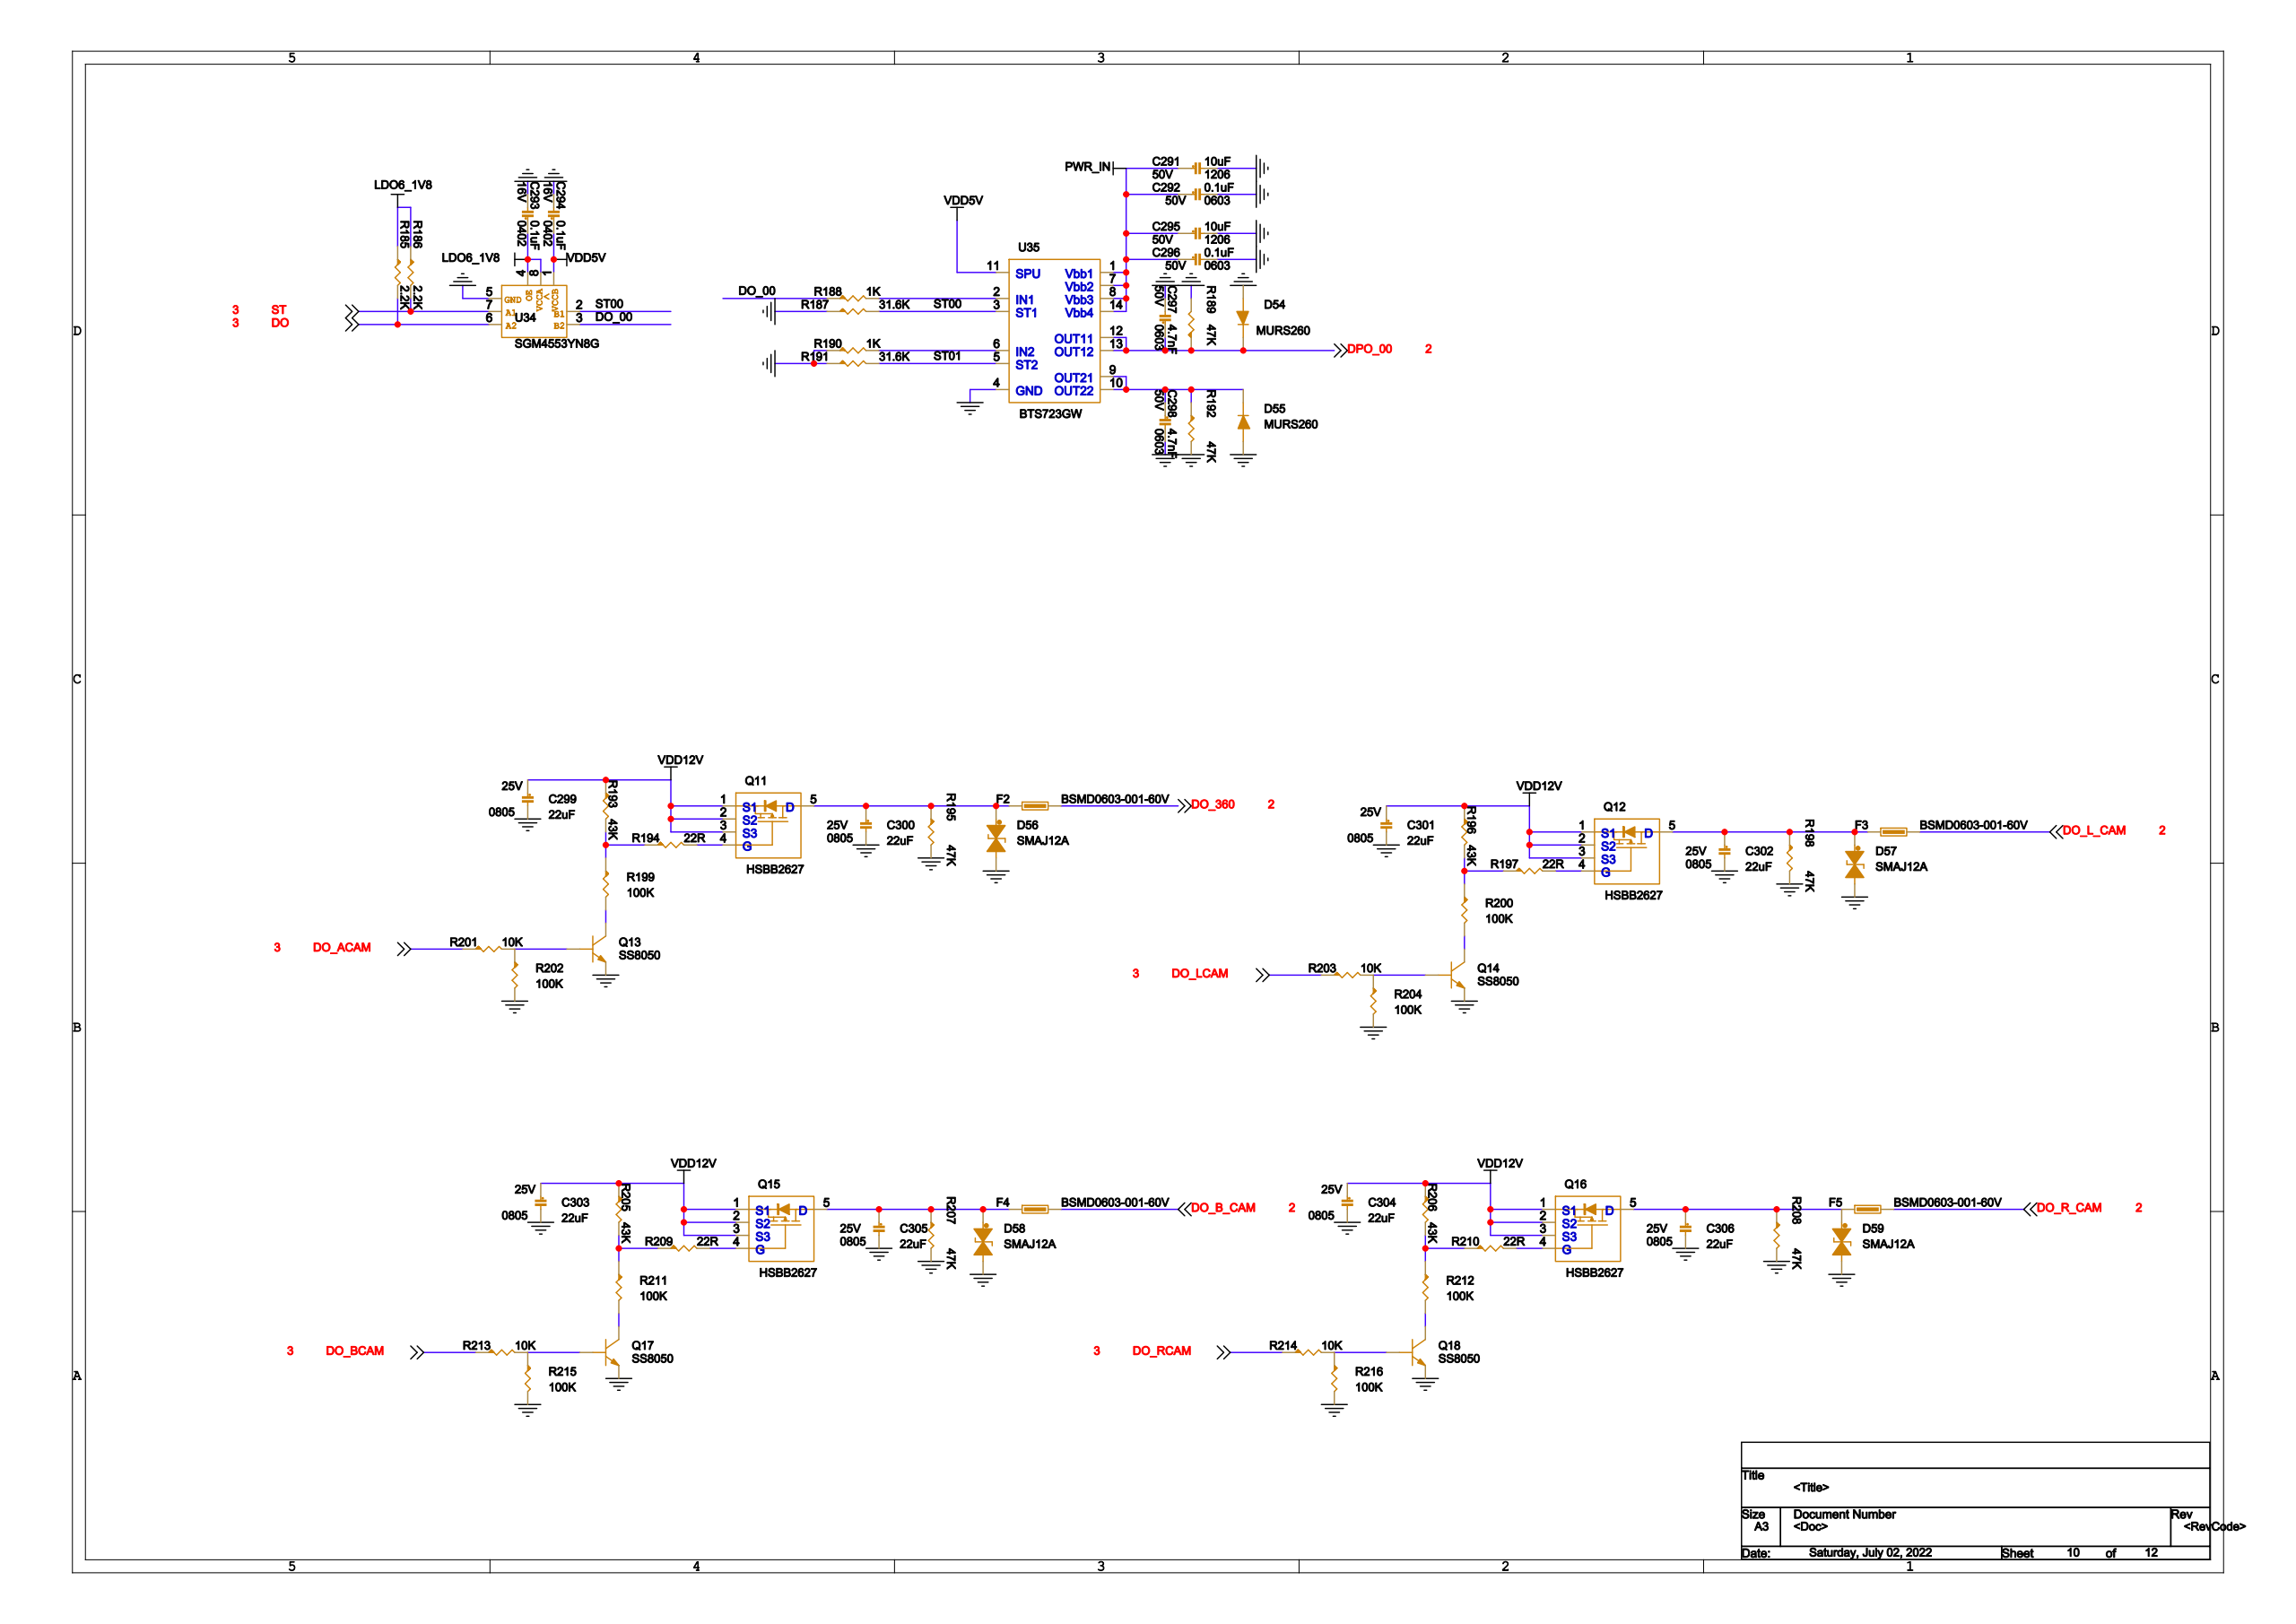Circuit board | Cadence Allegro | 970 parts | 627 nets | one sheet of the schematic
Parts on this sheet (reference | value | footprint):
C291 | 10uF | C1206
C292 | 0.1uF | C0603
C293 | 0.1uF | C0402
C294 | 0.1uF | C0402
C295 | 10uF | C1206
C296 | 0.1uF | C0603
C297 | 4.7nF | C0603
C298 | 4.7nF | C0603
C299 | 22uF | C0805
C300 | 22uF | C0805
C301 | 22uF | C0805
C302 | 22uF | C0805
C303 | 22uF | C0805
C304 | 22uF | C0805
C305 | 22uF | C0805
C306 | 22uF | C0805
D54 | MURS260 | SMA
D55 | MURS260 | SMA
D56 | SMAJ12A | SMA
D57 | SMAJ12A | SMA
D58 | SMAJ12A | SMA
D59 | SMAJ12A | SMA
F2 | BSMD0603-001-60V | R0603
F3 | BSMD0603-001-60V | R0603
F4 | BSMD0603-001-60V | R0603
F5 | BSMD0603-001-60V | R0603
Q11 | HSBB2627 | DFN3X3
Q12 | HSBB2627 | DFN3X3
Q13 | SS8050 | SOT-23
Q14 | SS8050 | SOT-23
Q15 | HSBB2627 | DFN3X3
Q16 | HSBB2627 | DFN3X3
Q17 | SS8050 | SOT-23
Q18 | SS8050 | SOT-23
R185 | 2.2K | R0402
R186 | 2.2K | R0402
R187 | 31.6K | R0402
R188 | 1K | R0402
R189 | 47K | R0805
R190 | 1K | R0402
R191 | 31.6K | R0402
R192 | 47K | R0805
R193 | 43K | R0402
R194 | 22R | R0402
R195 | 47K | R0805
R196 | 43K | R0402
R197 | 22R | R0402
R198 | 47K | R0805
R199 | 100K | R0402
R200 | 100K | R0402
R201 | 10K | R0402
R202 | 100K | R0402
R203 | 10K | R0402
R204 | 100K | R0402
R205 | 43K | R0402
R206 | 43K | R0402
R207 | 47K | R0805
R208 | 47K | R0805
R209 | 22R | R0402
R210 | 22R | R0402
R211 | 100K | R0402
R212 | 100K | R0402
R213 | 10K | R0402
R214 | 10K | R0402
R215 | 100K | R0402
R216 | 100K | R0402
U34 | SGM4553YN8G | SOT23_8
U35 | BTS723GW | SO14
Nets of these parts (net: part-pin ...):
VDD5V: C294-1 U34-1 U35-11
GND: C291-2 C292-2 C293-2 C294-2 C295-2 C296-2 C297-2 C298-2 C299-2 C300-2 C301-2 C302-2 C303-2 C304-2 C305-2 C306-2 D54-1 D55-1 D56-1 D57-1 D58-1 D59-1 Q13-2 Q14-2 Q17-2 Q18-2 R187-1 R189-2 R190-1 R191-1 R192-2 R195-2 R198-2 R202-2 R204-2 R207-2 R208-2 R215-2 R216-2 U34-5 U35-4
LDO6_1V8: C293-1 R185-1 R186-1 U34-4 U34-8
PWR_IN: C291-1 C292-1 C295-1 C296-1 U35-1 U35-7 U35-8 U35-14
VDD12V: C299-1 C301-1 C303-1 C304-1 Q11-1 Q11-2 Q11-3 Q12-1 Q12-2 Q12-3 Q15-1 Q15-2 Q15-3 Q16-1 Q16-2 Q16-3 R193-1 R196-1 R205-1 R206-1
DPO_00: C297-1 D54-2 R189-1 U35-12 U35-13
DO_B_CAM: F4-2
DO_L_CAM: F3-2
DO_360: F2-2
DO_R_CAM: F5-2
N19315440: R188-2 U35-2
N19315456: R190-2 U35-6
N19315989: C298-1 D55-2 R192-1 U35-9 U35-10
ST00: R187-2 U34-2 U35-3
ST01: R191-2 U35-5
N19342256: C300-1 D56-2 F2-1 Q11-5 R195-1
N19342555: C302-1 D57-2 F3-1 Q12-5 R198-1
N19342870: C305-1 D58-2 F4-1 Q15-5 R207-1
N19343201: C306-1 D59-2 F5-1 Q16-5 R208-1
N19342314: Q13-1 R201-2 R202-1
N19342336: Q13-3 R199-2
N19342613: Q14-1 R203-2 R204-1
N19342635: Q14-3 R200-2
N19342928: Q17-1 R213-2 R215-1
N19342950: Q17-3 R211-2
N19343259: Q18-1 R214-2 R216-1
N19343281: Q18-3 R212-2
N19342338: Q11-4 R194-2
N19342637: Q12-4 R197-2
N19342952: Q15-4 R209-2
N19343283: Q16-4 R210-2
N19342287: R193-2 R194-1 R199-1
N19342586: R196-2 R197-1 R200-1
N19342901: R205-2 R209-1 R211-1
N19343232: R206-2 R210-1 R212-1
DO_00: R188-1 U34-3
DO_ACAM: R201-1
DO_LCAM: R203-1
DO_BCAM: R213-1
DO_RCAM: R214-1
DO: R185-2 U34-6
ST: R186-2 U34-7